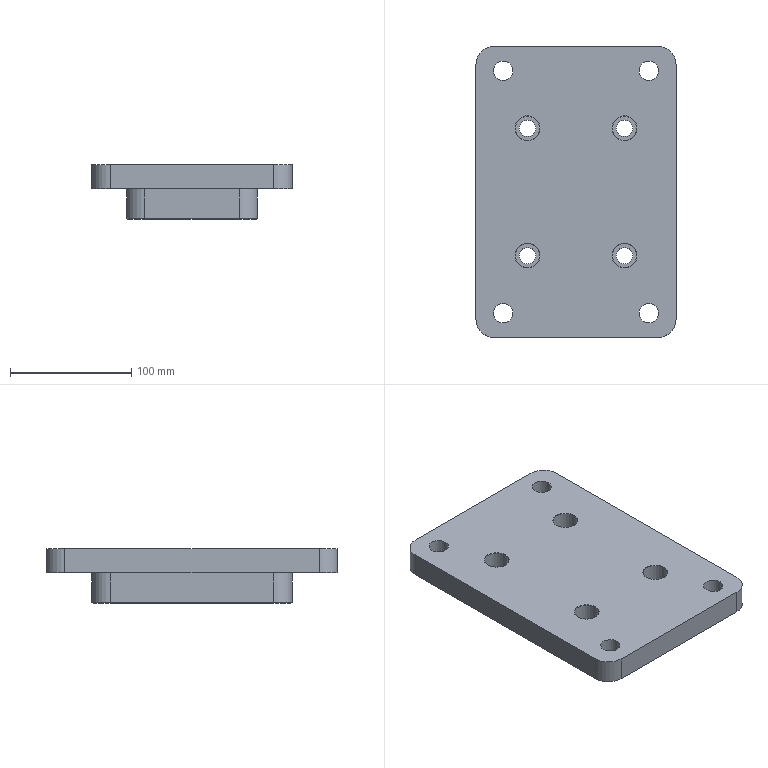NC program | NX | posted with a generic post | part box 165 x 240 x 45 mm
Lines 40 to 1182 of 5916:
(ZLEVEL_PROFILE_1_COPY , TOOL : D10)
N72 T10 M6
N74 G54
N76 G17 G0 G90 X-127.1 Y64.11 S3200 M3
N78 G43 Z30. H10
N80 Z1.78
N82 G94 G1 Z-0.22 F2200.
N84 X-125.599 Y64.978
N86 G3 X-125.099 Y65.845 R1.
N88 G1 X-125.1 Y67.177
N90 Y67.5
N92 G2 X-105. Y87.6 R20.1
N94 G1 X-104.677
N96 X-103.345 Y87.599
N98 G3 X-102.478 Y88.099 R1.
N100 G1 X-101.61 Y89.6
N102 Z1.78
N104 G0 Z30.
N106 Z1.56
N108 G1 Z-0.44
N110 X-102.478 Y88.099
N112 G2 X-103.345 Y87.599 R1.
N114 G1 X-104.677 Y87.6
N116 X-105.
N118 G3 X-125.1 Y67.5 R20.1
N120 G1 Y67.177
N122 X-125.099 Y65.845
N124 G2 X-125.599 Y64.978 R1.
N126 G1 X-127.1 Y64.11
N128 Z1.56
N130 G0 Z30.
N132 Z1.341
N134 G1 Z-0.659
N136 X-125.599 Y64.978
N138 G3 X-125.099 Y65.845 R1.
N140 G1 X-125.1 Y67.177
N142 Y67.5
N144 G2 X-105. Y87.6 R20.1
N146 G1 X-104.677
N148 X-103.345 Y87.599
N150 G3 X-102.478 Y88.099 R1.
N152 G1 X-101.61 Y89.6
N154 Z1.341
N156 G0 Z30.
N158 Z1.121
N160 G1 Z-0.879
N162 X-102.478 Y88.099
N164 G2 X-103.345 Y87.599 R1.
N166 G1 X-104.677 Y87.6
N168 X-105.
N170 G3 X-125.1 Y67.5 R20.1
N172 G1 Y67.177
N174 X-125.099 Y65.845
N176 G2 X-125.599 Y64.978 R1.
N178 G1 X-127.1 Y64.11
N180 Z1.121
N182 G0 Z30.
N184 Z0.901
N186 G1 Z-1.099
N188 X-125.599 Y64.978
N190 G3 X-125.099 Y65.845 R1.
N192 G1 X-125.1 Y67.177
N194 Y67.5
N196 G2 X-105. Y87.6 R20.1
N198 G1 X-104.677
N200 X-103.345 Y87.599
N202 G3 X-102.478 Y88.099 R1.
N204 G1 X-101.61 Y89.6
N206 Z0.901
N208 G0 Z30.
N210 Z0.681
N212 G1 Z-1.319
N214 X-102.478 Y88.099
N216 G2 X-103.345 Y87.599 R1.
N218 G1 X-104.677 Y87.6
N220 X-105.
N222 G3 X-125.1 Y67.5 R20.1
N224 G1 Y67.177
N226 X-125.099 Y65.845
N228 G2 X-125.599 Y64.978 R1.
N230 G1 X-127.1 Y64.11
N232 Z0.681
N234 G0 Z30.
N236 Z0.462
N238 G1 Z-1.538
N240 X-125.599 Y64.978
N242 G3 X-125.099 Y65.845 R1.
N244 G1 X-125.1 Y67.177
N246 Y67.5
N248 G2 X-105. Y87.6 R20.1
N250 G1 X-104.677
N252 X-103.345 Y87.599
N254 G3 X-102.478 Y88.099 R1.
N256 G1 X-101.61 Y89.6
N258 Z0.462
N260 G0 Z30.
N262 Z0.242
N264 G1 Z-1.758
N266 X-102.478 Y88.099
N268 G2 X-103.345 Y87.599 R1.
N270 G1 X-104.677 Y87.6
N272 X-105.
N274 G3 X-125.1 Y67.5 R20.1
N276 G1 Y67.177
N278 X-125.099 Y65.845
N280 G2 X-125.599 Y64.978 R1.
N282 G1 X-127.1 Y64.11
N284 Z0.242
N286 G0 Z30.
N288 Z0.022
N290 G1 Z-1.978
N292 X-125.599 Y64.978
N294 G3 X-125.099 Y65.845 R1.
N296 G1 X-125.1 Y67.177
N298 Y67.5
N300 G2 X-105. Y87.6 R20.1
N302 G1 X-104.677
N304 X-103.345 Y87.599
N306 G3 X-102.478 Y88.099 R1.
N308 G1 X-101.61 Y89.6
N310 Z0.022
N312 G0 Z30.
N314 Z-0.198
N316 G1 Z-2.198
N318 X-102.478 Y88.099
N320 G2 X-103.345 Y87.599 R1.
N322 G1 X-104.677 Y87.6
N324 X-105.
N326 G3 X-125.1 Y67.5 R20.1
N328 G1 Y67.177
N330 X-125.099 Y65.845
N332 G2 X-125.599 Y64.978 R1.
N334 G1 X-127.1 Y64.11
N336 Z-0.198
N338 G0 Z30.
N340 Z-0.418
N342 G1 Z-2.418
N344 X-125.599 Y64.978
N346 G3 X-125.099 Y65.845 R1.
N348 G1 X-125.1 Y67.177
N350 Y67.5
N352 G2 X-105. Y87.6 R20.1
N354 G1 X-104.677
N356 X-103.345 Y87.599
N358 G3 X-102.478 Y88.099 R1.
N360 G1 X-101.61 Y89.6
N362 Z-0.418
N364 G0 Z30.
N366 Z-0.637
N368 G1 Z-2.637
N370 X-102.478 Y88.099
N372 G2 X-103.345 Y87.599 R1.
N374 G1 X-104.677 Y87.6
N376 X-105.
N378 G3 X-125.1 Y67.5 R20.1
N380 G1 Y67.177
N382 X-125.099 Y65.845
N384 G2 X-125.599 Y64.978 R1.
N386 G1 X-127.1 Y64.11
N388 Z-0.637
N390 G0 Z30.
N392 Z-0.857
N394 G1 Z-2.857
N396 X-125.599 Y64.978
N398 G3 X-125.099 Y65.845 R1.
N400 G1 X-125.1 Y67.177
N402 Y67.5
N404 G2 X-105. Y87.6 R20.1
N406 G1 X-104.677
N408 X-103.345 Y87.599
N410 G3 X-102.478 Y88.099 R1.
N412 G1 X-101.61 Y89.6
N414 Z-0.857
N416 G0 Z30.
N418 Z-1.077
N420 G1 Z-3.077
N422 X-102.478 Y88.099
N424 G2 X-103.345 Y87.599 R1.
N426 G1 X-104.677 Y87.6
N428 X-105.
N430 G3 X-125.1 Y67.5 R20.1
N432 G1 Y67.177
N434 X-125.099 Y65.845
N436 G2 X-125.599 Y64.978 R1.
N438 G1 X-127.1 Y64.11
N440 Z-1.077
N442 G0 Z30.
N444 Z-1.297
N446 G1 Z-3.297
N448 X-125.599 Y64.978
N450 G3 X-125.099 Y65.845 R1.
N452 G1 X-125.1 Y67.177
N454 Y67.5
N456 G2 X-105. Y87.6 R20.1
N458 G1 X-104.677
N460 X-103.345 Y87.599
N462 G3 X-102.478 Y88.099 R1.
N464 G1 X-101.61 Y89.6
N466 Z-1.297
N468 G0 Z30.
N470 Z-1.516
N472 G1 Z-3.516
N474 X-102.478 Y88.099
N476 G2 X-103.345 Y87.599 R1.
N478 G1 X-104.677 Y87.6
N480 X-105.
N482 G3 X-125.1 Y67.5 R20.1
N484 G1 Y67.177
N486 X-125.099 Y65.845
N488 G2 X-125.599 Y64.978 R1.
N490 G1 X-127.1 Y64.11
N492 Z-1.516
N494 G0 Z30.
N496 Z-1.736
N498 G1 Z-3.736
N500 X-125.599 Y64.978
N502 G3 X-125.099 Y65.845 R1.
N504 G1 X-125.1 Y67.177
N506 Y67.5
N508 G2 X-105. Y87.6 R20.1
N510 G1 X-104.677
N512 X-103.345 Y87.599
N514 G3 X-102.478 Y88.099 R1.
N516 G1 X-101.61 Y89.6
N518 Z-1.736
N520 G0 Z30.
N522 Z-1.956
N524 G1 Z-3.956
N526 X-102.478 Y88.099
N528 G2 X-103.345 Y87.599 R1.
N530 G1 X-104.677 Y87.6
N532 X-105.
N534 G3 X-125.1 Y67.5 R20.1
N536 G1 Y67.177
N538 X-125.099 Y65.845
N540 G2 X-125.599 Y64.978 R1.
N542 G1 X-127.1 Y64.11
N544 Z-1.956
N546 G0 Z30.
N548 Z-2.176
N550 G1 Z-4.176
N552 X-125.599 Y64.978
N554 G3 X-125.099 Y65.845 R1.
N556 G1 X-125.1 Y67.177
N558 Y67.5
N560 G2 X-105. Y87.6 R20.1
N562 G1 X-104.677
N564 X-103.345 Y87.599
N566 G3 X-102.478 Y88.099 R1.
N568 G1 X-101.61 Y89.6
N570 Z-2.176
N572 G0 Z30.
N574 Z-2.396
N576 G1 Z-4.396
N578 X-102.478 Y88.099
N580 G2 X-103.345 Y87.599 R1.
N582 G1 X-104.677 Y87.6
N584 X-105.
N586 G3 X-125.1 Y67.5 R20.1
N588 G1 Y67.177
N590 X-125.099 Y65.845
N592 G2 X-125.599 Y64.978 R1.
N594 G1 X-127.1 Y64.11
N596 Z-2.396
N598 G0 Z30.
N600 Z-2.615
N602 G1 Z-4.615
N604 X-125.599 Y64.978
N606 G3 X-125.099 Y65.845 R1.
N608 G1 X-125.1 Y67.177
N610 Y67.5
N612 G2 X-105. Y87.6 R20.1
N614 G1 X-104.677
N616 X-103.345 Y87.599
N618 G3 X-102.478 Y88.099 R1.
N620 G1 X-101.61 Y89.6
N622 Z-2.615
N624 G0 Z30.
N626 Z-2.835
N628 G1 Z-4.835
N630 X-102.478 Y88.099
N632 G2 X-103.345 Y87.599 R1.
N634 G1 X-104.677 Y87.6
N636 X-105.
N638 G3 X-125.1 Y67.5 R20.1
N640 G1 Y67.177
N642 X-125.099 Y65.845
N644 G2 X-125.599 Y64.978 R1.
N646 G1 X-127.1 Y64.11
N648 Z-2.835
N650 G0 Z30.
N652 Z-3.055
N654 G1 Z-5.055
N656 X-125.599 Y64.978
N658 G3 X-125.099 Y65.845 R1.
N660 G1 X-125.1 Y67.177
N662 Y67.5
N664 G2 X-105. Y87.6 R20.1
N666 G1 X-104.677
N668 X-103.345 Y87.599
N670 G3 X-102.478 Y88.099 R1.
N672 G1 X-101.61 Y89.6
N674 Z-3.055
N676 G0 Z30.
N678 Z-3.275
N680 G1 Z-5.275
N682 X-102.478 Y88.099
N684 G2 X-103.345 Y87.599 R1.
N686 G1 X-104.677 Y87.6
N688 X-105.
N690 G3 X-125.1 Y67.5 R20.1
N692 G1 Y67.177
N694 X-125.099 Y65.845
N696 G2 X-125.599 Y64.978 R1.
N698 G1 X-127.1 Y64.11
N700 Z-3.275
N702 G0 Z30.
N704 Z-3.495
N706 G1 Z-5.495
N708 X-125.599 Y64.978
N710 G3 X-125.099 Y65.845 R1.
N712 G1 X-125.1 Y67.177
N714 Y67.5
N716 G2 X-105. Y87.6 R20.1
N718 G1 X-104.677
N720 X-103.345 Y87.599
N722 G3 X-102.478 Y88.099 R1.
N724 G1 X-101.61 Y89.6
N726 Z-3.495
N728 G0 Z30.
N730 Z-3.714
N732 G1 Z-5.714
N734 X-102.478 Y88.099
N736 G2 X-103.345 Y87.599 R1.
N738 G1 X-104.677 Y87.6
N740 X-105.
N742 G3 X-125.1 Y67.5 R20.1
N744 G1 Y67.177
N746 X-125.099 Y65.845
N748 G2 X-125.599 Y64.978 R1.
N750 G1 X-127.1 Y64.11
N752 Z-3.714
N754 G0 Z30.
N756 Z-3.934
N758 G1 Z-5.934
N760 X-125.599 Y64.978
N762 G3 X-125.099 Y65.845 R1.
N764 G1 X-125.1 Y67.177
N766 Y67.5
N768 G2 X-105. Y87.6 R20.1
N770 G1 X-104.677
N772 X-103.345 Y87.599
N774 G3 X-102.478 Y88.099 R1.
N776 G1 X-101.61 Y89.6
N778 Z-3.934
N780 G0 Z30.
N782 Z-4.154
N784 G1 Z-6.154
N786 X-102.478 Y88.099
N788 G2 X-103.345 Y87.599 R1.
N790 G1 X-104.677 Y87.6
N792 X-105.
N794 G3 X-125.1 Y67.5 R20.1
N796 G1 Y67.177
N798 X-125.099 Y65.845
N800 G2 X-125.599 Y64.978 R1.
N802 G1 X-127.1 Y64.11
N804 Z-4.154
N806 G0 Z30.
N808 Z-4.374
N810 G1 Z-6.374
N812 X-125.599 Y64.978
N814 G3 X-125.099 Y65.845 R1.
N816 G1 X-125.1 Y67.177
N818 Y67.5
N820 G2 X-105. Y87.6 R20.1
N822 G1 X-104.677
N824 X-103.345 Y87.599
N826 G3 X-102.478 Y88.099 R1.
N828 G1 X-101.61 Y89.6
N830 Z-4.374
N832 G0 Z30.
N834 Z-4.593
N836 G1 Z-6.593
N838 X-102.478 Y88.099
N840 G2 X-103.345 Y87.599 R1.
N842 G1 X-104.677 Y87.6
N844 X-105.
N846 G3 X-125.1 Y67.5 R20.1
N848 G1 Y67.177
N850 X-125.099 Y65.845
N852 G2 X-125.599 Y64.978 R1.
N854 G1 X-127.1 Y64.11
N856 Z-4.593
N858 G0 Z30.
N860 Z-4.813
N862 G1 Z-6.813
N864 X-125.599 Y64.978
N866 G3 X-125.099 Y65.845 R1.
N868 G1 X-125.1 Y67.177
N870 Y67.5
N872 G2 X-105. Y87.6 R20.1
N874 G1 X-104.677
N876 X-103.345 Y87.599
N878 G3 X-102.478 Y88.099 R1.
N880 G1 X-101.61 Y89.6
N882 Z-4.813
N884 G0 Z30.
N886 Z-5.033
N888 G1 Z-7.033
N890 X-102.478 Y88.099
N892 G2 X-103.345 Y87.599 R1.
N894 G1 X-104.677 Y87.6
N896 X-105.
N898 G3 X-125.1 Y67.5 R20.1
N900 G1 Y67.177
N902 X-125.099 Y65.845
N904 G2 X-125.599 Y64.978 R1.
N906 G1 X-127.1 Y64.11
N908 Z-5.033
N910 G0 Z30.
N912 Z-5.253
N914 G1 Z-7.253
N916 X-125.599 Y64.978
N918 G3 X-125.099 Y65.845 R1.
N920 G1 X-125.1 Y67.177
N922 Y67.5
N924 G2 X-105. Y87.6 R20.1
N926 G1 X-104.677
N928 X-103.345 Y87.599
N930 G3 X-102.478 Y88.099 R1.
N932 G1 X-101.61 Y89.6
N934 Z-5.253
N936 G0 Z30.
N938 Z-5.473
N940 G1 Z-7.473
N942 X-102.478 Y88.099
N944 G2 X-103.345 Y87.599 R1.
N946 G1 X-104.677 Y87.6
N948 X-105.
N950 G3 X-125.1 Y67.5 R20.1
N952 G1 Y67.177
N954 X-125.099 Y65.845
N956 G2 X-125.599 Y64.978 R1.
N958 G1 X-127.1 Y64.11
N960 Z-5.473
N962 G0 Z30.
N964 Z-5.692
N966 G1 Z-7.692
N968 X-125.599 Y64.978
N970 G3 X-125.099 Y65.845 R1.
N972 G1 X-125.1 Y67.177
N974 Y67.5
N976 G2 X-105. Y87.6 R20.1
N978 G1 X-104.677
N980 X-103.345 Y87.599
N982 G3 X-102.478 Y88.099 R1.
N984 G1 X-101.61 Y89.6
N986 Z-5.692
N988 G0 Z30.
N990 Z-5.912
N992 G1 Z-7.912
N994 X-102.478 Y88.099
N996 G2 X-103.345 Y87.599 R1.
N998 G1 X-104.677 Y87.6
N1000 X-105.
N1002 G3 X-125.1 Y67.5 R20.1
N1004 G1 Y67.177
N1006 X-125.099 Y65.845
N1008 G2 X-125.599 Y64.978 R1.
N1010 G1 X-127.1 Y64.11
N1012 Z-5.912
N1014 G0 Z30.
N1016 Z-6.132
N1018 G1 Z-8.132
N1020 X-125.599 Y64.978
N1022 G3 X-125.099 Y65.845 R1.
N1024 G1 X-125.1 Y67.177
N1026 Y67.5
N1028 G2 X-105. Y87.6 R20.1
N1030 G1 X-104.677
N1032 X-103.345 Y87.599
N1034 G3 X-102.478 Y88.099 R1.
N1036 G1 X-101.61 Y89.6
N1038 Z-6.132
N1040 G0 Z30.
N1042 Z-6.352
N1044 G1 Z-8.352
N1046 X-102.478 Y88.099
N1048 G2 X-103.345 Y87.599 R1.
N1050 G1 X-104.677 Y87.6
N1052 X-105.
N1054 G3 X-125.1 Y67.5 R20.1
N1056 G1 Y67.177
N1058 X-125.099 Y65.845
N1060 G2 X-125.599 Y64.978 R1.
N1062 G1 X-127.1 Y64.11
N1064 Z-6.352
N1066 G0 Z30.
N1068 Z-6.571
N1070 G1 Z-8.571
N1072 X-125.599 Y64.978
N1074 G3 X-125.099 Y65.845 R1.
N1076 G1 X-125.1 Y67.177
N1078 Y67.5
N1080 G2 X-105. Y87.6 R20.1
N1082 G1 X-104.677
N1084 X-103.345 Y87.599
N1086 G3 X-102.478 Y88.099 R1.
N1088 G1 X-101.61 Y89.6
N1090 Z-6.571
N1092 G0 Z30.
N1094 Z-6.791
N1096 G1 Z-8.791
N1098 X-102.478 Y88.099
N1100 G2 X-103.345 Y87.599 R1.
N1102 G1 X-104.677 Y87.6
N1104 X-105.
N1106 G3 X-125.1 Y67.5 R20.1
N1108 G1 Y67.177
N1110 X-125.099 Y65.845
N1112 G2 X-125.599 Y64.978 R1.
N1114 G1 X-127.1 Y64.11
N1116 Z-6.791
N1118 G0 Z30.
N1120 Z-7.011
N1122 G1 Z-9.011
N1124 X-125.599 Y64.978
N1126 G3 X-125.099 Y65.845 R1.
N1128 G1 X-125.1 Y67.177
N1130 Y67.5
N1132 G2 X-105. Y87.6 R20.1
N1134 G1 X-104.677
N1136 X-103.345 Y87.599
N1138 G3 X-102.478 Y88.099 R1.
N1140 G1 X-101.61 Y89.6
N1142 Z-7.011
N1144 G0 Z30.
N1146 Z-7.231
N1148 G1 Z-9.231
N1150 X-102.478 Y88.099
N1152 G2 X-103.345 Y87.599 R1.
N1154 G1 X-104.677 Y87.6
N1156 X-105.
N1158 G3 X-125.1 Y67.5 R20.1
N1160 G1 Y67.177
N1162 X-125.099 Y65.845
N1164 G2 X-125.599 Y64.978 R1.
N1166 G1 X-127.1 Y64.11
N1168 Z-7.231
N1170 G0 Z30.
N1172 Z-7.451
N1174 G1 Z-9.451
N1176 X-125.599 Y64.978
N1178 G3 X-125.099 Y65.845 R1.
N1180 G1 X-125.1 Y67.177
N1182 Y67.5
N1184 G2 X-105. Y87.6 R20.1
N1186 G1 X-104.677
N1188 X-103.345 Y87.599
N1190 G3 X-102.478 Y88.099 R1.
N1192 G1 X-101.61 Y89.6
N1194 Z-7.451
N1196 G0 Z30.
N1198 Z-7.67
N1200 G1 Z-9.67
N1202 X-102.478 Y88.099
N1204 G2 X-103.345 Y87.599 R1.
N1206 G1 X-104.677 Y87.6
N1208 X-105.
N1210 G3 X-125.1 Y67.5 R20.1
N1212 G1 Y67.177
N1214 X-125.099 Y65.845
N1216 G2 X-125.599 Y64.978 R1.
N1218 G1 X-127.1 Y64.11
N1220 Z-7.67
N1222 G0 Z30.
N1224 Z-7.89
N1226 G1 Z-9.89
N1228 X-125.599 Y64.978
N1230 G3 X-125.099 Y65.845 R1.
N1232 G1 X-125.1 Y67.177
N1234 Y67.5
N1236 G2 X-105. Y87.6 R20.1
N1238 G1 X-104.677
N1240 X-103.345 Y87.599
N1242 G3 X-102.478 Y88.099 R1.
N1244 G1 X-101.61 Y89.6
N1246 Z-7.89
N1248 G0 Z30.
N1250 Z-8.11
N1252 G1 Z-10.11
N1254 X-102.478 Y88.099
N1256 G2 X-103.345 Y87.599 R1.
N1258 G1 X-104.677 Y87.6
N1260 X-105.
N1262 G3 X-125.1 Y67.5 R20.1
N1264 G1 Y67.177
N1266 X-125.099 Y65.845
N1268 G2 X-125.599 Y64.978 R1.
N1270 G1 X-127.1 Y64.11
N1272 Z-8.11
N1274 G0 Z30.
N1276 Y64.111 Z-8.33
N1278 G1 Z-10.33
N1280 X-125.599 Y64.978
N1282 G3 X-125.099 Y65.845 R1.
N1284 G1 X-125.1 Y67.177
N1286 Y67.5
N1288 G2 X-105. Y87.6 R20.1
N1290 G1 X-104.677
N1292 X-103.345 Y87.599
N1294 G3 X-102.478 Y88.099 R1.
N1296 G1 X-101.611 Y89.6
N1298 Z-8.33
N1300 G0 Z30.
N1302 Z-8.549
N1304 G1 Z-10.549
N1306 X-102.478 Y88.099
N1308 G2 X-103.345 Y87.599 R1.
N1310 G1 X-104.677 Y87.6
N1312 X-105.
N1314 G3 X-125.1 Y67.5 R20.1
N1316 G1 Y67.177
N1318 X-125.099 Y65.845
N1320 G2 X-125.599 Y64.978 R1.
N1322 G1 X-127.1 Y64.111
N1324 Z-8.549
N1326 G0 Z30.
N1328 Z-8.769
N1330 G1 Z-10.769
N1332 X-125.599 Y64.978
N1334 G3 X-125.099 Y65.845 R1.
N1336 G1 X-125.1 Y67.177
N1338 Y67.5
N1340 G2 X-105. Y87.6 R20.1
N1342 G1 X-104.677
N1344 X-103.345 Y87.599
N1346 G3 X-102.478 Y88.099 R1.
N1348 G1 X-101.611 Y89.6
N1350 Z-8.769
N1352 G0 Z30.
N1354 Z-8.989
N1356 G1 Z-10.989
N1358 X-102.478 Y88.099
N1360 G2 X-103.345 Y87.599 R1.
N1362 G1 X-104.677 Y87.6
N1364 X-105.
N1366 G3 X-125.1 Y67.5 R20.1
N1368 G1 Y67.177
N1370 X-125.099 Y65.845
N1372 G2 X-125.599 Y64.978 R1.
N1374 G1 X-127.1 Y64.111
N1376 Z-8.989
N1378 G0 Z30.
N1380 Z-9.209
N1382 G1 Z-11.209
N1384 X-125.599 Y64.978
N1386 G3 X-125.099 Y65.845 R1.
N1388 G1 X-125.1 Y67.177
N1390 Y67.5
N1392 G2 X-105. Y87.6 R20.1
N1394 G1 X-104.677
N1396 X-103.345 Y87.599
N1398 G3 X-102.478 Y88.099 R1.
N1400 G1 X-101.611 Y89.6
N1402 Z-9.209
N1404 G0 Z30.
N1406 Z-9.429
N1408 G1 Z-11.429
N1410 X-102.478 Y88.099
N1412 G2 X-103.345 Y87.599 R1.
N1414 G1 X-104.677 Y87.6
N1416 X-105.
N1418 G3 X-125.1 Y67.5 R20.1
N1420 G1 Y67.177
N1422 X-125.099 Y65.845
N1424 G2 X-125.599 Y64.978 R1.
N1426 G1 X-127.1 Y64.111
N1428 Z-9.429
N1430 G0 Z30.
N1432 Z-9.648
N1434 G1 Z-11.648
N1436 X-125.599 Y64.978
N1438 G3 X-125.099 Y65.845 R1.
N1440 G1 X-125.1 Y67.177
N1442 Y67.5
N1444 G2 X-105. Y87.6 R20.1
N1446 G1 X-104.677
N1448 X-103.345 Y87.599
N1450 G3 X-102.478 Y88.099 R1.
N1452 G1 X-101.611 Y89.6
N1454 Z-9.648
N1456 G0 Z30.
N1458 Z-9.868
N1460 G1 Z-11.868
N1462 X-102.478 Y88.099
N1464 G2 X-103.345 Y87.599 R1.
N1466 G1 X-104.677 Y87.6
N1468 X-105.
N1470 G3 X-125.1 Y67.5 R20.1
N1472 G1 Y67.177
N1474 X-125.099 Y65.845
N1476 G2 X-125.599 Y64.978 R1.
N1478 G1 X-127.1 Y64.111
N1480 Z-9.868
N1482 G0 Z30.
N1484 Z-10.088
N1486 G1 Z-12.088
N1488 X-125.599 Y64.978
N1490 G3 X-125.099 Y65.845 R1.
N1492 G1 X-125.1 Y67.177
N1494 Y67.5
N1496 G2 X-105. Y87.6 R20.1
N1498 G1 X-104.677
N1500 X-103.345 Y87.599
N1502 G3 X-102.478 Y88.099 R1.
N1504 G1 X-101.611 Y89.6
N1506 Z-10.088
N1508 G0 Z30.
N1510 Z-10.308
N1512 G1 Z-12.308
N1514 X-102.478 Y88.099
N1516 G2 X-103.345 Y87.599 R1.
N1518 G1 X-104.677 Y87.6
N1520 X-105.
N1522 G3 X-125.1 Y67.5 R20.1
N1524 G1 Y67.177
N1526 X-125.099 Y65.845
N1528 G2 X-125.599 Y64.978 R1.
N1530 G1 X-127.1 Y64.111
N1532 Z-10.308
N1534 G0 Z30.
N1536 Z-10.527
N1538 G1 Z-12.527
N1540 X-125.599 Y64.978
N1542 G3 X-125.099 Y65.845 R1.
N1544 G1 X-125.1 Y67.177
N1546 Y67.5
N1548 G2 X-105. Y87.6 R20.1
N1550 G1 X-104.677
N1552 X-103.345 Y87.599
N1554 G3 X-102.478 Y88.099 R1.
N1556 G1 X-101.611 Y89.6
N1558 Z-10.527
N1560 G0 Z30.
N1562 Z-10.747
N1564 G1 Z-12.747
N1566 X-102.478 Y88.099
N1568 G2 X-103.345 Y87.599 R1.
N1570 G1 X-104.677 Y87.6
N1572 X-105.
N1574 G3 X-125.1 Y67.5 R20.1
N1576 G1 Y67.177
N1578 X-125.099 Y65.845
N1580 G2 X-125.599 Y64.978 R1.
N1582 G1 X-127.1 Y64.111
N1584 Z-10.747
N1586 G0 Z30.
N1588 Z-10.967
N1590 G1 Z-12.967
N1592 X-125.599 Y64.978
N1594 G3 X-125.099 Y65.845 R1.
N1596 G1 X-125.1 Y67.177
N1598 Y67.5
N1600 G2 X-105. Y87.6 R20.1
N1602 G1 X-104.677
N1604 X-103.345 Y87.599
N1606 G3 X-102.478 Y88.099 R1.
N1608 G1 X-101.611 Y89.6
N1610 Z-10.967
N1612 G0 Z30.
N1614 Z-11.187
N1616 G1 Z-13.187
N1618 X-102.478 Y88.099
N1620 G2 X-103.345 Y87.599 R1.
N1622 G1 X-104.677 Y87.6
N1624 X-105.
N1626 G3 X-125.1 Y67.5 R20.1
N1628 G1 Y67.177
N1630 X-125.099 Y65.845
N1632 G2 X-125.599 Y64.978 R1.
N1634 G1 X-127.1 Y64.111
N1636 Z-11.187
N1638 G0 Z30.
N1640 Z-11.407
N1642 G1 Z-13.407
N1644 X-125.599 Y64.978
N1646 G3 X-125.099 Y65.845 R1.
N1648 G1 X-125.1 Y67.177
N1650 Y67.5
N1652 G2 X-105. Y87.6 R20.1
N1654 G1 X-104.677
N1656 X-103.345 Y87.599
N1658 G3 X-102.478 Y88.099 R1.
N1660 G1 X-101.611 Y89.6
N1662 Z-11.407
N1664 G0 Z30.
N1666 Z-11.626
N1668 G1 Z-13.626
N1670 X-102.478 Y88.099
N1672 G2 X-103.345 Y87.599 R1.
N1674 G1 X-104.677 Y87.6
N1676 X-105.
N1678 G3 X-125.1 Y67.5 R20.1
N1680 G1 Y67.177
N1682 X-125.099 Y65.845
N1684 G2 X-125.599 Y64.978 R1.
N1686 G1 X-127.1 Y64.111
N1688 Z-11.626
N1690 G0 Z30.
N1692 Z-11.846
N1694 G1 Z-13.846
N1696 X-125.599 Y64.978
N1698 G3 X-125.099 Y65.845 R1.
N1700 G1 X-125.1 Y67.177
N1702 Y67.5
N1704 G2 X-105. Y87.6 R20.1
N1706 G1 X-104.677
N1708 X-103.345 Y87.599
N1710 G3 X-102.478 Y88.099 R1.
N1712 G1 X-101.611 Y89.6
N1714 Z-11.846
N1716 G0 Z30.
N1718 Z-12.066
N1720 G1 Z-14.066
N1722 X-102.478 Y88.099
N1724 G2 X-103.345 Y87.599 R1.
N1726 G1 X-104.677 Y87.6
N1728 X-105.
N1730 G3 X-125.1 Y67.5 R20.1
N1732 G1 Y67.177
N1734 X-125.099 Y65.845
N1736 G2 X-125.599 Y64.978 R1.
N1738 G1 X-127.1 Y64.111
N1740 Z-12.066
N1742 G0 Z30.
N1744 Z-12.286
N1746 G1 Z-14.286
N1748 X-125.599 Y64.978
N1750 G3 X-125.099 Y65.845 R1.
N1752 G1 X-125.1 Y67.177
N1754 Y67.5
N1756 G2 X-105. Y87.6 R20.1
N1758 G1 X-104.677
N1760 X-103.345 Y87.599
N1762 G3 X-102.478 Y88.099 R1.
N1764 G1 X-101.611 Y89.6
N1766 Z-12.286
N1768 G0 Z30.
N1770 Z-12.505
N1772 G1 Z-14.505
N1774 X-102.478 Y88.099
N1776 G2 X-103.345 Y87.599 R1.
N1778 G1 X-104.677 Y87.6
N1780 X-105.
N1782 G3 X-125.1 Y67.5 R20.1
N1784 G1 Y67.177
N1786 X-125.099 Y65.845
N1788 G2 X-125.599 Y64.978 R1.
N1790 G1 X-127.1 Y64.111
N1792 Z-12.505
N1794 G0 Z30.
N1796 Z-12.725
N1798 G1 Z-14.725
N1800 X-125.599 Y64.978
N1802 G3 X-125.099 Y65.845 R1.
N1804 G1 X-125.1 Y67.177
N1806 Y67.5
N1808 G2 X-105. Y87.6 R20.1
N1810 G1 X-104.677
N1812 X-103.345 Y87.599
N1814 G3 X-102.478 Y88.099 R1.
N1816 G1 X-101.611 Y89.6
N1818 Z-12.725
N1820 G0 Z30.
N1822 Z-12.945
N1824 G1 Z-14.945
N1826 X-102.478 Y88.099
N1828 G2 X-103.345 Y87.599 R1.
N1830 G1 X-104.677 Y87.6
N1832 X-105.
N1834 G3 X-125.1 Y67.5 R20.1
N1836 G1 Y67.177
N1838 X-125.099 Y65.845
N1840 G2 X-125.599 Y64.978 R1.
N1842 G1 X-127.1 Y64.111
N1844 Z-12.945
N1846 G0 Z30.
N1848 Z-13.165
N1850 G1 Z-15.165
N1852 X-125.599 Y64.978
N1854 G3 X-125.099 Y65.845 R1.
N1856 G1 X-125.1 Y67.177
N1858 Y67.5
N1860 G2 X-105. Y87.6 R20.1
N1862 G1 X-104.677
N1864 X-103.345 Y87.599
N1866 G3 X-102.478 Y88.099 R1.
N1868 G1 X-101.611 Y89.6
N1870 Z-13.165
N1872 G0 Z30.
N1874 Z-13.385
N1876 G1 Z-15.385
N1878 X-102.478 Y88.099
N1880 G2 X-103.345 Y87.599 R1.
N1882 G1 X-104.677 Y87.6
N1884 X-105.
N1886 G3 X-125.1 Y67.5 R20.1
N1888 G1 Y67.177
N1890 X-125.099 Y65.845
N1892 G2 X-125.599 Y64.978 R1.
N1894 G1 X-127.1 Y64.111
N1896 Z-13.385
N1898 G0 Z30.
N1900 Z-13.604
N1902 G1 Z-15.604
N1904 X-125.599 Y64.978
N1906 G3 X-125.099 Y65.845 R1.
N1908 G1 X-125.1 Y67.177
N1910 Y67.5
N1912 G2 X-105. Y87.6 R20.1
N1914 G1 X-104.677
N1916 X-103.345 Y87.599
N1918 G3 X-102.478 Y88.099 R1.
N1920 G1 X-101.611 Y89.6
N1922 Z-13.604
N1924 G0 Z30.
N1926 Z-13.824
N1928 G1 Z-15.824
N1930 X-102.478 Y88.099
N1932 G2 X-103.345 Y87.599 R1.
N1934 G1 X-104.677 Y87.6
N1936 X-105.
N1938 G3 X-125.1 Y67.5 R20.1
N1940 G1 Y67.177
N1942 X-125.099 Y65.845
N1944 G2 X-125.599 Y64.978 R1.
N1946 G1 X-127.1 Y64.111
N1948 Z-13.824
N1950 G0 Z30.
N1952 Z-14.044
N1954 G1 Z-16.044
N1956 X-125.599 Y64.978
N1958 G3 X-125.099 Y65.845 R1.
N1960 G1 X-125.1 Y67.177
N1962 Y67.5
N1964 G2 X-105. Y87.6 R20.1
N1966 G1 X-104.677
N1968 X-103.345 Y87.599
N1970 G3 X-102.478 Y88.099 R1.
N1972 G1 X-101.611 Y89.6
N1974 Z-14.044
N1976 G0 Z30.
N1978 Z-14.264
N1980 G1 Z-16.264
N1982 X-102.478 Y88.099
N1984 G2 X-103.345 Y87.599 R1.
N1986 G1 X-104.677 Y87.6
N1988 X-105.
N1990 G3 X-125.1 Y67.5 R20.1
N1992 G1 Y67.177
N1994 X-125.099 Y65.845
N1996 G2 X-125.599 Y64.978 R1.
N1998 G1 X-127.1 Y64.111
N2000 Z-14.264
N2002 G0 Z30.
N2004 Z-14.484
N2006 G1 Z-16.484
N2008 X-125.599 Y64.978
N2010 G3 X-125.099 Y65.845 R1.
N2012 G1 X-125.1 Y67.177
N2014 Y67.5
N2016 G2 X-105. Y87.6 R20.1
N2018 G1 X-104.677
N2020 X-103.345 Y87.599
N2022 G3 X-102.478 Y88.099 R1.
N2024 G1 X-101.611 Y89.6
N2026 Z-14.484
N2028 G0 Z30.
N2030 Z-14.703
N2032 G1 Z-16.703
N2034 X-102.478 Y88.099
N2036 G2 X-103.345 Y87.599 R1.
N2038 G1 X-104.677 Y87.6
N2040 X-105.
N2042 G3 X-125.1 Y67.5 R20.1
N2044 G1 Y67.177
N2046 X-125.099 Y65.845
N2048 G2 X-125.599 Y64.978 R1.
N2050 G1 X-127.1 Y64.111
N2052 Z-14.703
N2054 G0 Z30.
N2056 Z-14.923
N2058 G1 Z-16.923
N2060 X-125.599 Y64.978
N2062 G3 X-125.099 Y65.845 R1.
N2064 G1 X-125.1 Y67.177
N2066 Y67.5
N2068 G2 X-105. Y87.6 R20.1
N2070 G1 X-104.677
N2072 X-103.345 Y87.599
N2074 G3 X-102.478 Y88.099 R1.
N2076 G1 X-101.611 Y89.6
N2078 Z-14.923
N2080 G0 Z30.
N2082 Z-15.143
N2084 G1 Z-17.143
N2086 X-102.478 Y88.099
N2088 G2 X-103.345 Y87.599 R1.
N2090 G1 X-104.677 Y87.6
N2092 X-105.
N2094 G3 X-125.1 Y67.5 R20.1
N2096 G1 Y67.177
N2098 X-125.099 Y65.845
N2100 G2 X-125.599 Y64.978 R1.
N2102 G1 X-127.1 Y64.111
N2104 Z-15.143
N2106 G0 Z30.
N2108 Z-15.363
N2110 G1 Z-17.363
N2112 X-125.599 Y64.978
N2114 G3 X-125.099 Y65.845 R1.
N2116 G1 X-125.1 Y67.177
N2118 Y67.5
N2120 G2 X-105. Y87.6 R20.1
N2122 G1 X-104.677
N2124 X-103.345 Y87.599
N2126 G3 X-102.478 Y88.099 R1.
N2128 G1 X-101.611 Y89.6
N2130 Z-15.363
N2132 G0 Z30.
N2134 Z-15.582
N2136 G1 Z-17.582
N2138 X-102.478 Y88.099
N2140 G2 X-103.345 Y87.599 R1.
N2142 G1 X-104.677 Y87.6
N2144 X-105.
N2146 G3 X-125.1 Y67.5 R20.1
N2148 G1 Y67.177
N2150 X-125.099 Y65.845
N2152 G2 X-125.599 Y64.978 R1.
N2154 G1 X-127.1 Y64.111
N2156 Z-15.582
N2158 G0 Z30.
N2160 Z-15.802
N2162 G1 Z-17.802
N2164 X-125.599 Y64.978
N2166 G3 X-125.099 Y65.845 R1.
N2168 G1 X-125.1 Y67.177
N2170 Y67.5
N2172 G2 X-105. Y87.6 R20.1
N2174 G1 X-104.677
N2176 X-103.345 Y87.599
N2178 G3 X-102.478 Y88.099 R1.
N2180 G1 X-101.611 Y89.6
N2182 Z-15.802
N2184 G0 Z30.
N2186 Z-16.022
N2188 G1 Z-18.022
N2190 X-102.478 Y88.099
N2192 G2 X-103.345 Y87.599 R1.
N2194 G1 X-104.677 Y87.6
N2196 X-105.
N2198 G3 X-125.1 Y67.5 R20.1
N2200 G1 Y67.177
N2202 X-125.099 Y65.845
N2204 G2 X-125.599 Y64.978 R1.
N2206 G1 X-127.1 Y64.111
N2208 Z-16.022
N2210 G0 Z30.
N2212 Z-16.242
N2214 G1 Z-18.242
N2216 X-125.599 Y64.978
N2218 G3 X-125.099 Y65.845 R1.
N2220 G1 X-125.1 Y67.177
N2222 Y67.5
N2224 G2 X-105. Y87.6 R20.1
N2226 G1 X-104.677
N2228 X-103.345 Y87.599
N2230 G3 X-102.478 Y88.099 R1.
N2232 G1 X-101.611 Y89.6
N2234 Z-16.242
N2236 G0 Z30.
N2238 Z-16.462
N2240 G1 Z-18.462
N2242 X-102.478 Y88.099
N2244 G2 X-103.345 Y87.599 R1.
N2246 G1 X-104.677 Y87.6
N2248 X-105.
N2250 G3 X-125.1 Y67.5 R20.1
N2252 G1 Y67.177
N2254 X-125.099 Y65.845
N2256 G2 X-125.599 Y64.978 R1.
N2258 G1 X-127.1 Y64.111
N2260 Z-16.462
N2262 G0 Z30.
N2264 Z-16.681
N2266 G1 Z-18.681
N2268 X-125.599 Y64.978
N2270 G3 X-125.099 Y65.845 R1.
N2272 G1 X-125.1 Y67.177
N2274 Y67.5
N2276 G2 X-105. Y87.6 R20.1
N2278 G1 X-104.677
N2280 X-103.345 Y87.599
N2282 G3 X-102.478 Y88.099 R1.
N2284 G1 X-101.611 Y89.6
N2286 Z-16.681
N2288 G0 Z30.
N2290 Z-16.901
N2292 G1 Z-18.901
N2294 X-102.478 Y88.099
N2296 G2 X-103.345 Y87.599 R1.
N2298 G1 X-104.677 Y87.6
N2300 X-105.
N2302 G3 X-125.1 Y67.5 R20.1
N2304 G1 Y67.177
N2306 X-125.099 Y65.845
N2308 G2 X-125.599 Y64.978 R1.
N2310 G1 X-127.1 Y64.111
N2312 Z-16.901
N2314 G0 Z30.
N2316 Z-17.121
N2318 G1 Z-19.121
N2320 X-125.599 Y64.978
N2322 G3 X-125.099 Y65.845 R1.
N2324 G1 X-125.1 Y67.177
N2326 Y67.5
N2328 G2 X-105. Y87.6 R20.1
N2330 G1 X-104.677
N2332 X-103.345 Y87.599
N2334 G3 X-102.478 Y88.099 R1.
N2336 G1 X-101.611 Y89.6
N2338 Z-17.121
N2340 G0 Z30.
N2342 Z-17.341
N2344 G1 Z-19.341
N2346 X-102.478 Y88.099
N2348 G2 X-103.345 Y87.599 R1.
N2350 G1 X-104.677 Y87.6